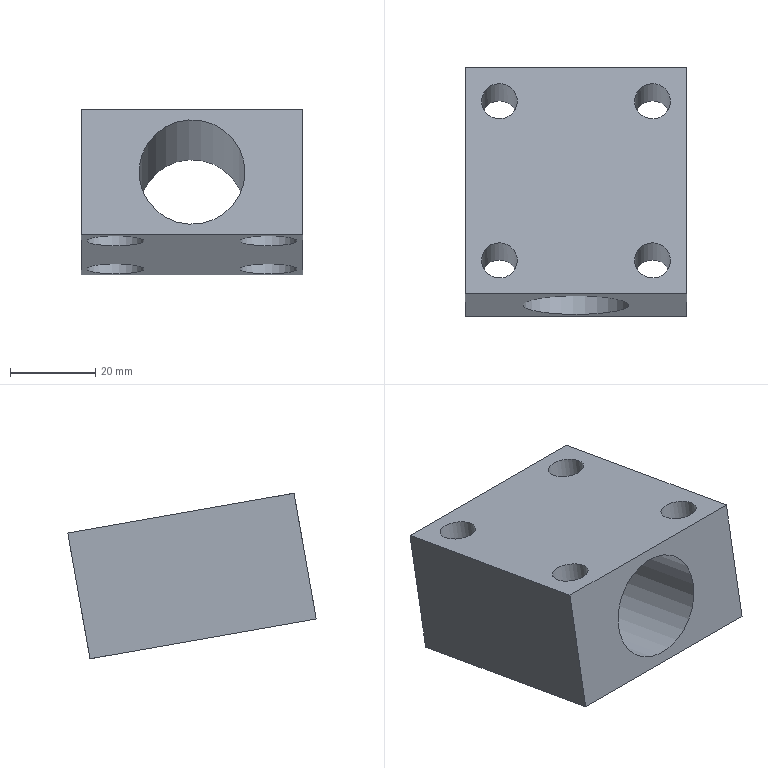Part | NX | features MAIN_BODY 2 | 1 solid | 19 faces | box 52 x 58.389 x 38.921 mm | volume 48838 mm3 | plane 10 | cylinder 9 | commonest cylinder face diameters 8.4 x4 13.5 x4 24.9 x1
STEP:
#1=CARTESIAN_POINT('',(586.25,-782.616,24.815));
#2=VERTEX_POINT('',#1);
#3=CARTESIAN_POINT('',(579.5,-782.616,24.815));
#4=DIRECTION('',(0.,-0.1736,-0.9848));
#5=DIRECTION('',(1.,0.,0.));
#6=AXIS2_PLACEMENT_3D('',#3,#4,#5);
#7=CIRCLE('',#6,6.75);
#8=EDGE_CURVE('',#2,#2,#7,.T.);
#9=ORIENTED_EDGE('',*,*,#8,.F.);
#10=EDGE_LOOP('',(#9));
#11=FACE_BOUND('',#10,.T.);
#12=CARTESIAN_POINT('',(550.25,-820.038,31.414));
#13=VERTEX_POINT('',#12);
#14=CARTESIAN_POINT('',(543.5,-820.038,31.414));
#15=DIRECTION('',(0.,-0.1736,-0.9848));
#16=DIRECTION('',(1.,0.,0.));
#17=AXIS2_PLACEMENT_3D('',#14,#15,#16);
#18=CIRCLE('',#17,6.75);
#19=EDGE_CURVE('',#13,#13,#18,.T.);
#20=ORIENTED_EDGE('',*,*,#19,.F.);
#21=EDGE_LOOP('',(#20));
#22=FACE_BOUND('',#21,.T.);
#23=CARTESIAN_POINT('',(587.5,-827.917,32.803));
#24=VERTEX_POINT('',#23);
#25=CARTESIAN_POINT('',(535.5,-827.917,32.803));
#26=VERTEX_POINT('',#25);
#27=CARTESIAN_POINT('',(587.5,-827.917,32.803));
#28=DIRECTION('',(-1.,0.,0.));
#29=VECTOR('',#28,1000.);
#30=LINE('',#27,#29);
#31=EDGE_CURVE('',#24,#26,#30,.T.);
#32=ORIENTED_EDGE('',*,*,#31,.T.);
#33=CARTESIAN_POINT('',(535.5,-774.737,23.426));
#34=VERTEX_POINT('',#33);
#35=CARTESIAN_POINT('',(535.5,-774.737,23.426));
#36=DIRECTION('',(0.,-0.9848,0.1736));
#37=VECTOR('',#36,1000.);
#38=LINE('',#35,#37);
#39=EDGE_CURVE('',#34,#26,#38,.T.);
#40=ORIENTED_EDGE('',*,*,#39,.F.);
#41=CARTESIAN_POINT('',(587.5,-774.737,23.426));
#42=VERTEX_POINT('',#41);
#43=CARTESIAN_POINT('',(587.5,-774.737,23.426));
#44=DIRECTION('',(-1.,0.,0.));
#45=VECTOR('',#44,1000.);
#46=LINE('',#43,#45);
#47=EDGE_CURVE('',#42,#34,#46,.T.);
#48=ORIENTED_EDGE('',*,*,#47,.F.);
#49=CARTESIAN_POINT('',(587.5,-774.737,23.426));
#50=DIRECTION('',(0.,-0.9848,0.1736));
#51=VECTOR('',#50,1000.);
#52=LINE('',#49,#51);
#53=EDGE_CURVE('',#42,#24,#52,.T.);
#54=ORIENTED_EDGE('',*,*,#53,.T.);
#55=EDGE_LOOP('',(#32,#40,#48,#54));
#56=FACE_BOUND('',#55,.T.);
#57=CARTESIAN_POINT('',(550.25,-782.616,24.815));
#58=VERTEX_POINT('',#57);
#59=CARTESIAN_POINT('',(543.5,-782.616,24.815));
#60=DIRECTION('',(0.,-0.1736,-0.9848));
#61=DIRECTION('',(1.,0.,0.));
#62=AXIS2_PLACEMENT_3D('',#59,#60,#61);
#63=CIRCLE('',#62,6.75);
#64=EDGE_CURVE('',#58,#58,#63,.T.);
#65=ORIENTED_EDGE('',*,*,#64,.F.);
#66=EDGE_LOOP('',(#65));
#67=FACE_BOUND('',#66,.T.);
#68=CARTESIAN_POINT('',(586.25,-820.038,31.414));
#69=VERTEX_POINT('',#68);
#70=CARTESIAN_POINT('',(579.5,-820.038,31.414));
#71=DIRECTION('',(0.,-0.1736,-0.9848));
#72=DIRECTION('',(1.,0.,0.));
#73=AXIS2_PLACEMENT_3D('',#70,#71,#72);
#74=CIRCLE('',#73,6.75);
#75=EDGE_CURVE('',#69,#69,#74,.T.);
#76=ORIENTED_EDGE('',*,*,#75,.F.);
#77=EDGE_LOOP('',(#76));
#78=FACE_BOUND('',#77,.T.);
#79=CARTESIAN_POINT('',(587.5,-774.737,23.426));
#80=DIRECTION('',(0.,0.1736,0.9848));
#81=DIRECTION('',(-1.,0.,0.));
#82=AXIS2_PLACEMENT_3D('',#79,#80,#81);
#83=PLANE('',#82);
#84=ADVANCED_FACE('',(#11,#22,#56,#67,#78),#83,.F.);
#85=CARTESIAN_POINT('',(583.7,-814.829,60.958));
#86=VERTEX_POINT('',#85);
#87=CARTESIAN_POINT('',(579.5,-814.829,60.958));
#88=DIRECTION('',(0.,-0.1736,-0.9848));
#89=DIRECTION('',(1.,0.,0.));
#90=AXIS2_PLACEMENT_3D('',#87,#88,#89);
#91=CIRCLE('',#90,4.2);
#92=EDGE_CURVE('',#86,#86,#91,.T.);
#93=ORIENTED_EDGE('',*,*,#92,.F.);
#94=EDGE_LOOP('',(#93));
#95=FACE_BOUND('',#94,.T.);
#96=CARTESIAN_POINT('',(579.5,-814.687,37.578));
#97=VERTEX_POINT('',#96);
#98=CARTESIAN_POINT('',(579.5,-818.823,38.307));
#99=DIRECTION('',(0.,-0.1736,-0.9848));
#100=DIRECTION('',(0.,0.9848,-0.1736));
#101=AXIS2_PLACEMENT_3D('',#98,#99,#100);
#102=CIRCLE('',#101,4.2);
#103=EDGE_CURVE('',#97,#97,#102,.F.);
#104=ORIENTED_EDGE('',*,*,#103,.F.);
#105=EDGE_LOOP('',(#104));
#106=FACE_BOUND('',#105,.T.);
#107=CARTESIAN_POINT('',(579.5,-814.829,60.958));
#108=DIRECTION('',(0.,-0.1736,-0.9848));
#109=DIRECTION('',(0.,0.9848,-0.1736));
#110=AXIS2_PLACEMENT_3D('',#107,#108,#109);
#111=CYLINDRICAL_SURFACE('',#110,4.2);
#112=ADVANCED_FACE('',(#95,#106),#111,.F.);
#113=CARTESIAN_POINT('',(583.7,-777.406,54.359));
#114=VERTEX_POINT('',#113);
#115=CARTESIAN_POINT('',(579.5,-777.406,54.359));
#116=DIRECTION('',(0.,-0.1736,-0.9848));
#117=DIRECTION('',(1.,0.,0.));
#118=AXIS2_PLACEMENT_3D('',#115,#116,#117);
#119=CIRCLE('',#118,4.2);
#120=EDGE_CURVE('',#114,#114,#119,.T.);
#121=ORIENTED_EDGE('',*,*,#120,.F.);
#122=EDGE_LOOP('',(#121));
#123=FACE_BOUND('',#122,.T.);
#124=CARTESIAN_POINT('',(579.5,-777.264,30.98));
#125=VERTEX_POINT('',#124);
#126=CARTESIAN_POINT('',(579.5,-781.4,31.709));
#127=DIRECTION('',(0.,-0.1736,-0.9848));
#128=DIRECTION('',(0.,0.9848,-0.1736));
#129=AXIS2_PLACEMENT_3D('',#126,#127,#128);
#130=CIRCLE('',#129,4.2);
#131=EDGE_CURVE('',#125,#125,#130,.F.);
#132=ORIENTED_EDGE('',*,*,#131,.F.);
#133=EDGE_LOOP('',(#132));
#134=FACE_BOUND('',#133,.T.);
#135=CARTESIAN_POINT('',(579.5,-777.406,54.359));
#136=DIRECTION('',(0.,-0.1736,-0.9848));
#137=DIRECTION('',(0.,0.9848,-0.1736));
#138=AXIS2_PLACEMENT_3D('',#135,#136,#137);
#139=CYLINDRICAL_SURFACE('',#138,4.2);
#140=ADVANCED_FACE('',(#123,#134),#139,.F.);
#141=CARTESIAN_POINT('',(547.7,-777.406,54.359));
#142=VERTEX_POINT('',#141);
#143=CARTESIAN_POINT('',(543.5,-777.406,54.359));
#144=DIRECTION('',(0.,-0.1736,-0.9848));
#145=DIRECTION('',(1.,0.,0.));
#146=AXIS2_PLACEMENT_3D('',#143,#144,#145);
#147=CIRCLE('',#146,4.2);
#148=EDGE_CURVE('',#142,#142,#147,.T.);
#149=ORIENTED_EDGE('',*,*,#148,.F.);
#150=EDGE_LOOP('',(#149));
#151=FACE_BOUND('',#150,.T.);
#152=CARTESIAN_POINT('',(543.5,-777.264,30.98));
#153=VERTEX_POINT('',#152);
#154=CARTESIAN_POINT('',(543.5,-781.4,31.709));
#155=DIRECTION('',(0.,-0.1736,-0.9848));
#156=DIRECTION('',(0.,0.9848,-0.1736));
#157=AXIS2_PLACEMENT_3D('',#154,#155,#156);
#158=CIRCLE('',#157,4.2);
#159=EDGE_CURVE('',#153,#153,#158,.F.);
#160=ORIENTED_EDGE('',*,*,#159,.F.);
#161=EDGE_LOOP('',(#160));
#162=FACE_BOUND('',#161,.T.);
#163=CARTESIAN_POINT('',(543.5,-777.406,54.359));
#164=DIRECTION('',(0.,-0.1736,-0.9848));
#165=DIRECTION('',(0.,0.9848,-0.1736));
#166=AXIS2_PLACEMENT_3D('',#163,#164,#165);
#167=CYLINDRICAL_SURFACE('',#166,4.2);
#168=ADVANCED_FACE('',(#151,#162),#167,.F.);
#169=CARTESIAN_POINT('',(535.5,-822.707,62.347));
#170=VERTEX_POINT('',#169);
#171=CARTESIAN_POINT('',(535.5,-827.917,32.803));
#172=DIRECTION('',(0.,0.1736,0.9848));
#173=VECTOR('',#172,1000.);
#174=LINE('',#171,#173);
#175=EDGE_CURVE('',#26,#170,#174,.T.);
#176=ORIENTED_EDGE('',*,*,#175,.T.);
#177=CARTESIAN_POINT('',(535.5,-769.528,52.97));
#178=VERTEX_POINT('',#177);
#179=CARTESIAN_POINT('',(535.5,-769.528,52.97));
#180=DIRECTION('',(0.,-0.9848,0.1736));
#181=VECTOR('',#180,1000.);
#182=LINE('',#179,#181);
#183=EDGE_CURVE('',#178,#170,#182,.T.);
#184=ORIENTED_EDGE('',*,*,#183,.F.);
#185=CARTESIAN_POINT('',(535.5,-774.737,23.426));
#186=DIRECTION('',(0.,0.1736,0.9848));
#187=VECTOR('',#186,1000.);
#188=LINE('',#185,#187);
#189=EDGE_CURVE('',#34,#178,#188,.T.);
#190=ORIENTED_EDGE('',*,*,#189,.F.);
#191=ORIENTED_EDGE('',*,*,#39,.T.);
#192=EDGE_LOOP('',(#176,#184,#190,#191));
#193=FACE_BOUND('',#192,.T.);
#194=CARTESIAN_POINT('',(535.5,-774.737,23.426));
#195=DIRECTION('',(1.,0.,0.));
#196=DIRECTION('',(0.,0.1736,0.9848));
#197=AXIS2_PLACEMENT_3D('',#194,#195,#196);
#198=PLANE('',#197);
#199=ADVANCED_FACE('',(#193),#198,.F.);
#200=ORIENTED_EDGE('',*,*,#92,.T.);
#201=EDGE_LOOP('',(#200));
#202=FACE_BOUND('',#201,.T.);
#203=ORIENTED_EDGE('',*,*,#120,.T.);
#204=EDGE_LOOP('',(#203));
#205=FACE_BOUND('',#204,.T.);
#206=CARTESIAN_POINT('',(547.7,-814.829,60.958));
#207=VERTEX_POINT('',#206);
#208=CARTESIAN_POINT('',(543.5,-814.829,60.958));
#209=DIRECTION('',(0.,-0.1736,-0.9848));
#210=DIRECTION('',(1.,0.,0.));
#211=AXIS2_PLACEMENT_3D('',#208,#209,#210);
#212=CIRCLE('',#211,4.2);
#213=EDGE_CURVE('',#207,#207,#212,.T.);
#214=ORIENTED_EDGE('',*,*,#213,.T.);
#215=EDGE_LOOP('',(#214));
#216=FACE_BOUND('',#215,.T.);
#217=ORIENTED_EDGE('',*,*,#148,.T.);
#218=EDGE_LOOP('',(#217));
#219=FACE_BOUND('',#218,.T.);
#220=CARTESIAN_POINT('',(587.5,-822.707,62.347));
#221=VERTEX_POINT('',#220);
#222=CARTESIAN_POINT('',(535.5,-822.707,62.347));
#223=DIRECTION('',(1.,0.,0.));
#224=VECTOR('',#223,1000.);
#225=LINE('',#222,#224);
#226=EDGE_CURVE('',#170,#221,#225,.T.);
#227=ORIENTED_EDGE('',*,*,#226,.T.);
#228=CARTESIAN_POINT('',(587.5,-769.528,52.97));
#229=VERTEX_POINT('',#228);
#230=CARTESIAN_POINT('',(587.5,-769.528,52.97));
#231=DIRECTION('',(0.,-0.9848,0.1736));
#232=VECTOR('',#231,1000.);
#233=LINE('',#230,#232);
#234=EDGE_CURVE('',#229,#221,#233,.T.);
#235=ORIENTED_EDGE('',*,*,#234,.F.);
#236=CARTESIAN_POINT('',(535.5,-769.528,52.97));
#237=DIRECTION('',(1.,0.,0.));
#238=VECTOR('',#237,1000.);
#239=LINE('',#236,#238);
#240=EDGE_CURVE('',#178,#229,#239,.T.);
#241=ORIENTED_EDGE('',*,*,#240,.F.);
#242=ORIENTED_EDGE('',*,*,#183,.T.);
#243=EDGE_LOOP('',(#227,#235,#241,#242));
#244=FACE_BOUND('',#243,.T.);
#245=CARTESIAN_POINT('',(535.5,-769.528,52.97));
#246=DIRECTION('',(0.,-0.1736,-0.9848));
#247=DIRECTION('',(0.,0.9848,-0.1736));
#248=AXIS2_PLACEMENT_3D('',#245,#246,#247);
#249=PLANE('',#248);
#250=ADVANCED_FACE('',(#202,#205,#216,#219,#244),#249,.F.);
#251=CARTESIAN_POINT('',(587.5,-822.707,62.347));
#252=DIRECTION('',(0.,-0.1736,-0.9848));
#253=VECTOR('',#252,1000.);
#254=LINE('',#251,#253);
#255=EDGE_CURVE('',#221,#24,#254,.T.);
#256=ORIENTED_EDGE('',*,*,#255,.T.);
#257=ORIENTED_EDGE('',*,*,#53,.F.);
#258=CARTESIAN_POINT('',(587.5,-769.528,52.97));
#259=DIRECTION('',(0.,-0.1736,-0.9848));
#260=VECTOR('',#259,1000.);
#261=LINE('',#258,#260);
#262=EDGE_CURVE('',#229,#42,#261,.T.);
#263=ORIENTED_EDGE('',*,*,#262,.F.);
#264=ORIENTED_EDGE('',*,*,#234,.T.);
#265=EDGE_LOOP('',(#256,#257,#263,#264));
#266=FACE_BOUND('',#265,.T.);
#267=CARTESIAN_POINT('',(587.5,-769.528,52.97));
#268=DIRECTION('',(-1.,0.,0.));
#269=DIRECTION('',(0.,-0.1736,-0.9848));
#270=AXIS2_PLACEMENT_3D('',#267,#268,#269);
#271=PLANE('',#270);
#272=ADVANCED_FACE('',(#266),#271,.F.);
#273=CARTESIAN_POINT('',(573.95,-772.132,38.198));
#274=VERTEX_POINT('',#273);
#275=CARTESIAN_POINT('',(561.5,-772.132,38.198));
#276=DIRECTION('',(0.,-0.9848,0.1736));
#277=DIRECTION('',(1.,0.,0.));
#278=AXIS2_PLACEMENT_3D('',#275,#276,#277);
#279=CIRCLE('',#278,12.45);
#280=EDGE_CURVE('',#274,#274,#279,.T.);
#281=ORIENTED_EDGE('',*,*,#280,.F.);
#282=EDGE_LOOP('',(#281));
#283=FACE_BOUND('',#282,.T.);
#284=CARTESIAN_POINT('',(573.95,-825.312,47.575));
#285=VERTEX_POINT('',#284);
#286=CARTESIAN_POINT('',(561.5,-825.312,47.575));
#287=DIRECTION('',(0.,-0.9848,0.1736));
#288=DIRECTION('',(1.,0.,0.));
#289=AXIS2_PLACEMENT_3D('',#286,#287,#288);
#290=CIRCLE('',#289,12.45);
#291=EDGE_CURVE('',#285,#285,#290,.T.);
#292=ORIENTED_EDGE('',*,*,#291,.T.);
#293=EDGE_LOOP('',(#292));
#294=FACE_BOUND('',#293,.T.);
#295=CARTESIAN_POINT('',(561.5,-772.132,38.198));
#296=DIRECTION('',(0.,-0.9848,0.1736));
#297=DIRECTION('',(1.,0.,0.));
#298=AXIS2_PLACEMENT_3D('',#295,#296,#297);
#299=CYLINDRICAL_SURFACE('',#298,12.45);
#300=ADVANCED_FACE('',(#283,#294),#299,.F.);
#301=ORIENTED_EDGE('',*,*,#47,.T.);
#302=ORIENTED_EDGE('',*,*,#189,.T.);
#303=ORIENTED_EDGE('',*,*,#240,.T.);
#304=ORIENTED_EDGE('',*,*,#262,.T.);
#305=EDGE_LOOP('',(#301,#302,#303,#304));
#306=FACE_BOUND('',#305,.T.);
#307=ORIENTED_EDGE('',*,*,#280,.T.);
#308=EDGE_LOOP('',(#307));
#309=FACE_BOUND('',#308,.T.);
#310=CARTESIAN_POINT('',(535.5,-774.737,23.426));
#311=DIRECTION('',(0.,0.9848,-0.1736));
#312=DIRECTION('',(-1.,0.,0.));
#313=AXIS2_PLACEMENT_3D('',#310,#311,#312);
#314=PLANE('',#313);
#315=ADVANCED_FACE('',(#306,#309),#314,.T.);
#316=ORIENTED_EDGE('',*,*,#31,.F.);
#317=ORIENTED_EDGE('',*,*,#255,.F.);
#318=ORIENTED_EDGE('',*,*,#226,.F.);
#319=ORIENTED_EDGE('',*,*,#175,.F.);
#320=EDGE_LOOP('',(#316,#317,#318,#319));
#321=FACE_BOUND('',#320,.T.);
#322=ORIENTED_EDGE('',*,*,#291,.F.);
#323=EDGE_LOOP('',(#322));
#324=FACE_BOUND('',#323,.T.);
#325=CARTESIAN_POINT('',(535.5,-827.917,32.803));
#326=DIRECTION('',(0.,0.9848,-0.1736));
#327=DIRECTION('',(-1.,0.,0.));
#328=AXIS2_PLACEMENT_3D('',#325,#326,#327);
#329=PLANE('',#328);
#330=ADVANCED_FACE('',(#321,#324),#329,.F.);
#331=ORIENTED_EDGE('',*,*,#19,.T.);
#332=EDGE_LOOP('',(#331));
#333=FACE_BOUND('',#332,.T.);
#334=CARTESIAN_POINT('',(550.25,-818.823,38.307));
#335=VERTEX_POINT('',#334);
#336=CARTESIAN_POINT('',(543.5,-818.823,38.307));
#337=DIRECTION('',(0.,-0.1736,-0.9848));
#338=DIRECTION('',(1.,0.,0.));
#339=AXIS2_PLACEMENT_3D('',#336,#337,#338);
#340=CIRCLE('',#339,6.75);
#341=EDGE_CURVE('',#335,#335,#340,.T.);
#342=ORIENTED_EDGE('',*,*,#341,.F.);
#343=EDGE_LOOP('',(#342));
#344=FACE_BOUND('',#343,.T.);
#345=CARTESIAN_POINT('',(543.5,-820.038,31.414));
#346=DIRECTION('',(0.,0.1736,0.9848));
#347=DIRECTION('',(0.,-0.9848,0.1736));
#348=AXIS2_PLACEMENT_3D('',#345,#346,#347);
#349=CYLINDRICAL_SURFACE('',#348,6.75);
#350=ADVANCED_FACE('',(#333,#344),#349,.F.);
#351=CARTESIAN_POINT('',(543.5,-814.687,37.578));
#352=VERTEX_POINT('',#351);
#353=CARTESIAN_POINT('',(543.5,-818.823,38.307));
#354=DIRECTION('',(0.,-0.1736,-0.9848));
#355=DIRECTION('',(0.,0.9848,-0.1736));
#356=AXIS2_PLACEMENT_3D('',#353,#354,#355);
#357=CIRCLE('',#356,4.2);
#358=EDGE_CURVE('',#352,#352,#357,.T.);
#359=ORIENTED_EDGE('',*,*,#358,.F.);
#360=EDGE_LOOP('',(#359));
#361=FACE_BOUND('',#360,.T.);
#362=ORIENTED_EDGE('',*,*,#341,.T.);
#363=EDGE_LOOP('',(#362));
#364=FACE_BOUND('',#363,.T.);
#365=CARTESIAN_POINT('',(543.5,-818.823,38.307));
#366=DIRECTION('',(0.,-0.1736,-0.9848));
#367=DIRECTION('',(0.,0.9848,-0.1736));
#368=AXIS2_PLACEMENT_3D('',#365,#366,#367);
#369=PLANE('',#368);
#370=ADVANCED_FACE('',(#361,#364),#369,.T.);
#371=ORIENTED_EDGE('',*,*,#358,.T.);
#372=EDGE_LOOP('',(#371));
#373=FACE_BOUND('',#372,.T.);
#374=ORIENTED_EDGE('',*,*,#213,.F.);
#375=EDGE_LOOP('',(#374));
#376=FACE_BOUND('',#375,.T.);
#377=CARTESIAN_POINT('',(543.5,-814.829,60.958));
#378=DIRECTION('',(0.,-0.1736,-0.9848));
#379=DIRECTION('',(0.,0.9848,-0.1736));
#380=AXIS2_PLACEMENT_3D('',#377,#378,#379);
#381=CYLINDRICAL_SURFACE('',#380,4.2);
#382=ADVANCED_FACE('',(#373,#376),#381,.F.);
#383=CARTESIAN_POINT('',(550.25,-781.4,31.709));
#384=VERTEX_POINT('',#383);
#385=CARTESIAN_POINT('',(543.5,-781.4,31.709));
#386=DIRECTION('',(0.,-0.1736,-0.9848));
#387=DIRECTION('',(1.,0.,0.));
#388=AXIS2_PLACEMENT_3D('',#385,#386,#387);
#389=CIRCLE('',#388,6.75);
#390=EDGE_CURVE('',#384,#384,#389,.T.);
#391=ORIENTED_EDGE('',*,*,#390,.T.);
#392=EDGE_LOOP('',(#391));
#393=FACE_BOUND('',#392,.T.);
#394=ORIENTED_EDGE('',*,*,#159,.T.);
#395=EDGE_LOOP('',(#394));
#396=FACE_BOUND('',#395,.T.);
#397=CARTESIAN_POINT('',(543.5,-781.4,31.709));
#398=DIRECTION('',(0.,-0.1736,-0.9848));
#399=DIRECTION('',(0.,0.9848,-0.1736));
#400=AXIS2_PLACEMENT_3D('',#397,#398,#399);
#401=PLANE('',#400);
#402=ADVANCED_FACE('',(#393,#396),#401,.T.);
#403=ORIENTED_EDGE('',*,*,#64,.T.);
#404=EDGE_LOOP('',(#403));
#405=FACE_BOUND('',#404,.T.);
#406=ORIENTED_EDGE('',*,*,#390,.F.);
#407=EDGE_LOOP('',(#406));
#408=FACE_BOUND('',#407,.T.);
#409=CARTESIAN_POINT('',(543.5,-782.616,24.815));
#410=DIRECTION('',(0.,0.1736,0.9848));
#411=DIRECTION('',(0.,-0.9848,0.1736));
#412=AXIS2_PLACEMENT_3D('',#409,#410,#411);
#413=CYLINDRICAL_SURFACE('',#412,6.75);
#414=ADVANCED_FACE('',(#405,#408),#413,.F.);
#415=CARTESIAN_POINT('',(586.25,-781.4,31.709));
#416=VERTEX_POINT('',#415);
#417=CARTESIAN_POINT('',(579.5,-781.4,31.709));
#418=DIRECTION('',(0.,-0.1736,-0.9848));
#419=DIRECTION('',(1.,0.,0.));
#420=AXIS2_PLACEMENT_3D('',#417,#418,#419);
#421=CIRCLE('',#420,6.75);
#422=EDGE_CURVE('',#416,#416,#421,.T.);
#423=ORIENTED_EDGE('',*,*,#422,.T.);
#424=EDGE_LOOP('',(#423));
#425=FACE_BOUND('',#424,.T.);
#426=ORIENTED_EDGE('',*,*,#131,.T.);
#427=EDGE_LOOP('',(#426));
#428=FACE_BOUND('',#427,.T.);
#429=CARTESIAN_POINT('',(579.5,-781.4,31.709));
#430=DIRECTION('',(0.,-0.1736,-0.9848));
#431=DIRECTION('',(0.,0.9848,-0.1736));
#432=AXIS2_PLACEMENT_3D('',#429,#430,#431);
#433=PLANE('',#432);
#434=ADVANCED_FACE('',(#425,#428),#433,.T.);
#435=ORIENTED_EDGE('',*,*,#8,.T.);
#436=EDGE_LOOP('',(#435));
#437=FACE_BOUND('',#436,.T.);
#438=ORIENTED_EDGE('',*,*,#422,.F.);
#439=EDGE_LOOP('',(#438));
#440=FACE_BOUND('',#439,.T.);
#441=CARTESIAN_POINT('',(579.5,-782.616,24.815));
#442=DIRECTION('',(0.,0.1736,0.9848));
#443=DIRECTION('',(0.,-0.9848,0.1736));
#444=AXIS2_PLACEMENT_3D('',#441,#442,#443);
#445=CYLINDRICAL_SURFACE('',#444,6.75);
#446=ADVANCED_FACE('',(#437,#440),#445,.F.);
#447=CARTESIAN_POINT('',(586.25,-818.823,38.307));
#448=VERTEX_POINT('',#447);
#449=CARTESIAN_POINT('',(579.5,-818.823,38.307));
#450=DIRECTION('',(0.,-0.1736,-0.9848));
#451=DIRECTION('',(1.,0.,0.));
#452=AXIS2_PLACEMENT_3D('',#449,#450,#451);
#453=CIRCLE('',#452,6.75);
#454=EDGE_CURVE('',#448,#448,#453,.T.);
#455=ORIENTED_EDGE('',*,*,#454,.T.);
#456=EDGE_LOOP('',(#455));
#457=FACE_BOUND('',#456,.T.);
#458=ORIENTED_EDGE('',*,*,#103,.T.);
#459=EDGE_LOOP('',(#458));
#460=FACE_BOUND('',#459,.T.);
#461=CARTESIAN_POINT('',(579.5,-818.823,38.307));
#462=DIRECTION('',(0.,-0.1736,-0.9848));
#463=DIRECTION('',(0.,0.9848,-0.1736));
#464=AXIS2_PLACEMENT_3D('',#461,#462,#463);
#465=PLANE('',#464);
#466=ADVANCED_FACE('',(#457,#460),#465,.T.);
#467=ORIENTED_EDGE('',*,*,#75,.T.);
#468=EDGE_LOOP('',(#467));
#469=FACE_BOUND('',#468,.T.);
#470=ORIENTED_EDGE('',*,*,#454,.F.);
#471=EDGE_LOOP('',(#470));
#472=FACE_BOUND('',#471,.T.);
#473=CARTESIAN_POINT('',(579.5,-820.038,31.414));
#474=DIRECTION('',(0.,0.1736,0.9848));
#475=DIRECTION('',(0.,-0.9848,0.1736));
#476=AXIS2_PLACEMENT_3D('',#473,#474,#475);
#477=CYLINDRICAL_SURFACE('',#476,6.75);
#478=ADVANCED_FACE('',(#469,#472),#477,.F.);
#479=CLOSED_SHELL('',(#84,#112,#140,#168,#199,#250,#272,#300,#315,#330,#350,#370,#382,#402,#414,#434,#446,#466,#478));
#480=MANIFOLD_SOLID_BREP('',#479);
#481=(LENGTH_UNIT()NAMED_UNIT(*)SI_UNIT(.MILLI.,.METRE.));
#482=UNCERTAINTY_MEASURE_WITH_UNIT(LENGTH_MEASURE(0.00001),#481,'','');
#483=(NAMED_UNIT(*)PLANE_ANGLE_UNIT()SI_UNIT($,.RADIAN.));
#484=(NAMED_UNIT(*)SI_UNIT($,.STERADIAN.)SOLID_ANGLE_UNIT());
#485=(GEOMETRIC_REPRESENTATION_CONTEXT(3)GLOBAL_UNCERTAINTY_ASSIGNED_CONTEXT((#482))GLOBAL_UNIT_ASSIGNED_CONTEXT((#481,#483,#484))REPRESENTATION_CONTEXT('',''));
#486=ADVANCED_BREP_SHAPE_REPRESENTATION('',(#480),#485);